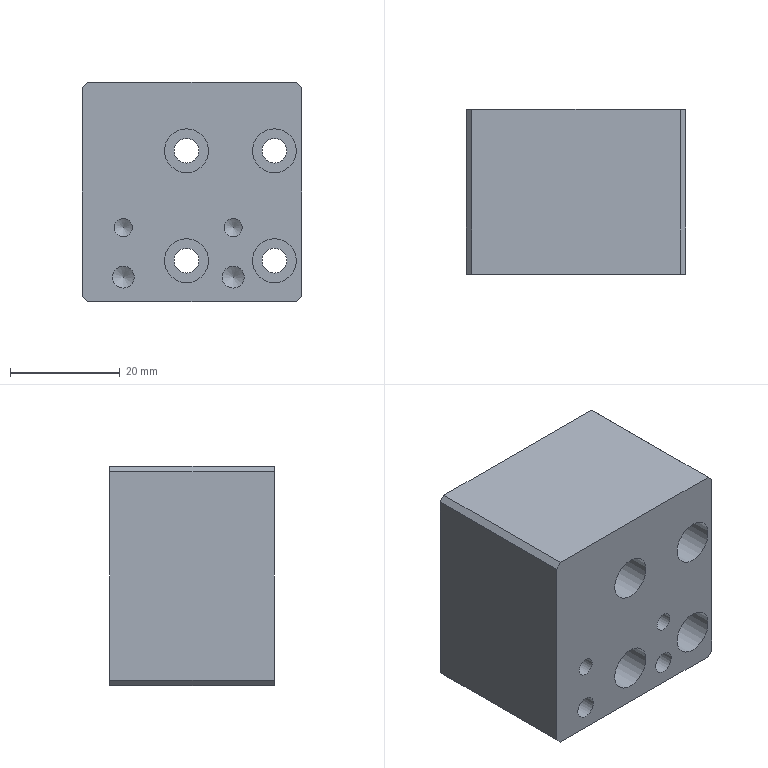Part | NX | 1 solid | 30 faces | box 40 x 30 x 40 mm | volume 42153 mm3 | plane 14 | cylinder 12 | cone 4 | commonest cylinder face diameters 4.5 x4 8 x4 3.3 x2 4 x2
STEP:
#1=CARTESIAN_POINT('',(-19.,30.,-20.));
#2=VERTEX_POINT('',#1);
#3=CARTESIAN_POINT('',(-20.,30.,-19.));
#4=VERTEX_POINT('',#3);
#5=CARTESIAN_POINT('',(-20.,30.,-19.));
#6=DIRECTION('',(-0.7071,0.,0.7071));
#7=VECTOR('',#6,1000.);
#8=LINE('',#5,#7);
#9=EDGE_CURVE('',#2,#4,#8,.T.);
#10=ORIENTED_EDGE('',*,*,#9,.F.);
#11=CARTESIAN_POINT('',(-19.,0.,-20.));
#12=VERTEX_POINT('',#11);
#13=CARTESIAN_POINT('',(-19.,30.,-20.));
#14=DIRECTION('',(0.,1.,0.));
#15=VECTOR('',#14,1000.);
#16=LINE('',#13,#15);
#17=EDGE_CURVE('',#12,#2,#16,.T.);
#18=ORIENTED_EDGE('',*,*,#17,.F.);
#19=CARTESIAN_POINT('',(-20.,0.,-19.));
#20=VERTEX_POINT('',#19);
#21=CARTESIAN_POINT('',(-19.5,0.,-19.5));
#22=DIRECTION('',(0.7071,0.,-0.7071));
#23=VECTOR('',#22,1000.);
#24=LINE('',#21,#23);
#25=EDGE_CURVE('',#20,#12,#24,.T.);
#26=ORIENTED_EDGE('',*,*,#25,.F.);
#27=CARTESIAN_POINT('',(-20.,30.,-19.));
#28=DIRECTION('',(0.,-1.,0.));
#29=VECTOR('',#28,1000.);
#30=LINE('',#27,#29);
#31=EDGE_CURVE('',#4,#20,#30,.T.);
#32=ORIENTED_EDGE('',*,*,#31,.F.);
#33=EDGE_LOOP('',(#10,#18,#26,#32));
#34=FACE_BOUND('',#33,.T.);
#35=CARTESIAN_POINT('',(-20.,30.,-19.));
#36=DIRECTION('',(0.7071,0.,0.7071));
#37=DIRECTION('',(0.,-1.,0.));
#38=AXIS2_PLACEMENT_3D('',#35,#36,#37);
#39=PLANE('',#38);
#40=ADVANCED_FACE('',(#34),#39,.F.);
#41=CARTESIAN_POINT('',(-20.,30.,19.));
#42=VERTEX_POINT('',#41);
#43=CARTESIAN_POINT('',(-19.,30.,20.));
#44=VERTEX_POINT('',#43);
#45=CARTESIAN_POINT('',(-19.,30.,20.));
#46=DIRECTION('',(0.7071,0.,0.7071));
#47=VECTOR('',#46,1000.);
#48=LINE('',#45,#47);
#49=EDGE_CURVE('',#42,#44,#48,.T.);
#50=ORIENTED_EDGE('',*,*,#49,.F.);
#51=CARTESIAN_POINT('',(-20.,0.,19.));
#52=VERTEX_POINT('',#51);
#53=CARTESIAN_POINT('',(-20.,30.,19.));
#54=DIRECTION('',(0.,1.,0.));
#55=VECTOR('',#54,1000.);
#56=LINE('',#53,#55);
#57=EDGE_CURVE('',#52,#42,#56,.T.);
#58=ORIENTED_EDGE('',*,*,#57,.F.);
#59=CARTESIAN_POINT('',(-19.,0.,20.));
#60=VERTEX_POINT('',#59);
#61=CARTESIAN_POINT('',(-19.5,0.,19.5));
#62=DIRECTION('',(-0.7071,0.,-0.7071));
#63=VECTOR('',#62,1000.);
#64=LINE('',#61,#63);
#65=EDGE_CURVE('',#60,#52,#64,.T.);
#66=ORIENTED_EDGE('',*,*,#65,.F.);
#67=CARTESIAN_POINT('',(-19.,30.,20.));
#68=DIRECTION('',(0.,-1.,0.));
#69=VECTOR('',#68,1000.);
#70=LINE('',#67,#69);
#71=EDGE_CURVE('',#44,#60,#70,.T.);
#72=ORIENTED_EDGE('',*,*,#71,.F.);
#73=EDGE_LOOP('',(#50,#58,#66,#72));
#74=FACE_BOUND('',#73,.T.);
#75=CARTESIAN_POINT('',(-19.,30.,20.));
#76=DIRECTION('',(0.7071,0.,-0.7071));
#77=DIRECTION('',(0.,-1.,0.));
#78=AXIS2_PLACEMENT_3D('',#75,#76,#77);
#79=PLANE('',#78);
#80=ADVANCED_FACE('',(#74),#79,.F.);
#81=CARTESIAN_POINT('',(19.,30.,20.));
#82=VERTEX_POINT('',#81);
#83=CARTESIAN_POINT('',(20.,30.,19.));
#84=VERTEX_POINT('',#83);
#85=CARTESIAN_POINT('',(20.,30.,19.));
#86=DIRECTION('',(0.7071,0.,-0.7071));
#87=VECTOR('',#86,1000.);
#88=LINE('',#85,#87);
#89=EDGE_CURVE('',#82,#84,#88,.T.);
#90=ORIENTED_EDGE('',*,*,#89,.F.);
#91=CARTESIAN_POINT('',(19.,0.,20.));
#92=VERTEX_POINT('',#91);
#93=CARTESIAN_POINT('',(19.,30.,20.));
#94=DIRECTION('',(0.,1.,0.));
#95=VECTOR('',#94,1000.);
#96=LINE('',#93,#95);
#97=EDGE_CURVE('',#92,#82,#96,.T.);
#98=ORIENTED_EDGE('',*,*,#97,.F.);
#99=CARTESIAN_POINT('',(20.,0.,19.));
#100=VERTEX_POINT('',#99);
#101=CARTESIAN_POINT('',(19.5,0.,19.5));
#102=DIRECTION('',(-0.7071,0.,0.7071));
#103=VECTOR('',#102,1000.);
#104=LINE('',#101,#103);
#105=EDGE_CURVE('',#100,#92,#104,.T.);
#106=ORIENTED_EDGE('',*,*,#105,.F.);
#107=CARTESIAN_POINT('',(20.,30.,19.));
#108=DIRECTION('',(0.,-1.,0.));
#109=VECTOR('',#108,1000.);
#110=LINE('',#107,#109);
#111=EDGE_CURVE('',#84,#100,#110,.T.);
#112=ORIENTED_EDGE('',*,*,#111,.F.);
#113=EDGE_LOOP('',(#90,#98,#106,#112));
#114=FACE_BOUND('',#113,.T.);
#115=CARTESIAN_POINT('',(20.,30.,19.));
#116=DIRECTION('',(-0.7071,0.,-0.7071));
#117=DIRECTION('',(0.,-1.,0.));
#118=AXIS2_PLACEMENT_3D('',#115,#116,#117);
#119=PLANE('',#118);
#120=ADVANCED_FACE('',(#114),#119,.F.);
#121=CARTESIAN_POINT('',(20.,30.,-19.));
#122=VERTEX_POINT('',#121);
#123=CARTESIAN_POINT('',(19.,30.,-20.));
#124=VERTEX_POINT('',#123);
#125=CARTESIAN_POINT('',(19.,30.,-20.));
#126=DIRECTION('',(-0.7071,0.,-0.7071));
#127=VECTOR('',#126,1000.);
#128=LINE('',#125,#127);
#129=EDGE_CURVE('',#122,#124,#128,.T.);
#130=ORIENTED_EDGE('',*,*,#129,.F.);
#131=CARTESIAN_POINT('',(20.,0.,-19.));
#132=VERTEX_POINT('',#131);
#133=CARTESIAN_POINT('',(20.,30.,-19.));
#134=DIRECTION('',(0.,1.,0.));
#135=VECTOR('',#134,1000.);
#136=LINE('',#133,#135);
#137=EDGE_CURVE('',#132,#122,#136,.T.);
#138=ORIENTED_EDGE('',*,*,#137,.F.);
#139=CARTESIAN_POINT('',(19.,0.,-20.));
#140=VERTEX_POINT('',#139);
#141=CARTESIAN_POINT('',(19.5,0.,-19.5));
#142=DIRECTION('',(0.7071,0.,0.7071));
#143=VECTOR('',#142,1000.);
#144=LINE('',#141,#143);
#145=EDGE_CURVE('',#140,#132,#144,.T.);
#146=ORIENTED_EDGE('',*,*,#145,.F.);
#147=CARTESIAN_POINT('',(19.,30.,-20.));
#148=DIRECTION('',(0.,-1.,0.));
#149=VECTOR('',#148,1000.);
#150=LINE('',#147,#149);
#151=EDGE_CURVE('',#124,#140,#150,.T.);
#152=ORIENTED_EDGE('',*,*,#151,.F.);
#153=EDGE_LOOP('',(#130,#138,#146,#152));
#154=FACE_BOUND('',#153,.T.);
#155=CARTESIAN_POINT('',(19.,30.,-20.));
#156=DIRECTION('',(-0.7071,0.,0.7071));
#157=DIRECTION('',(0.,-1.,0.));
#158=AXIS2_PLACEMENT_3D('',#155,#156,#157);
#159=PLANE('',#158);
#160=ADVANCED_FACE('',(#154),#159,.F.);
#161=CARTESIAN_POINT('',(15.,25.,-16.5));
#162=VERTEX_POINT('',#161);
#163=CARTESIAN_POINT('',(15.,25.,-12.5));
#164=DIRECTION('',(0.,-1.,0.));
#165=DIRECTION('',(0.,0.,-1.));
#166=AXIS2_PLACEMENT_3D('',#163,#164,#165);
#167=CIRCLE('',#166,4.);
#168=EDGE_CURVE('',#162,#162,#167,.T.);
#169=ORIENTED_EDGE('',*,*,#168,.T.);
#170=EDGE_LOOP('',(#169));
#171=FACE_BOUND('',#170,.T.);
#172=CARTESIAN_POINT('',(15.,25.,-14.75));
#173=VERTEX_POINT('',#172);
#174=CARTESIAN_POINT('',(15.,25.,-12.5));
#175=DIRECTION('',(0.,-1.,0.));
#176=DIRECTION('',(0.,0.,-1.));
#177=AXIS2_PLACEMENT_3D('',#174,#175,#176);
#178=CIRCLE('',#177,2.25);
#179=EDGE_CURVE('',#173,#173,#178,.T.);
#180=ORIENTED_EDGE('',*,*,#179,.F.);
#181=EDGE_LOOP('',(#180));
#182=FACE_BOUND('',#181,.T.);
#183=CARTESIAN_POINT('',(17.25,25.,-12.5));
#184=DIRECTION('',(0.,1.,0.));
#185=DIRECTION('',(0.,0.,1.));
#186=AXIS2_PLACEMENT_3D('',#183,#184,#185);
#187=PLANE('',#186);
#188=ADVANCED_FACE('',(#171,#182),#187,.F.);
#189=CARTESIAN_POINT('',(-1.,25.,-8.5));
#190=VERTEX_POINT('',#189);
#191=CARTESIAN_POINT('',(-1.,25.,-12.5));
#192=DIRECTION('',(0.,-1.,0.));
#193=DIRECTION('',(0.,0.,1.));
#194=AXIS2_PLACEMENT_3D('',#191,#192,#193);
#195=CIRCLE('',#194,4.);
#196=EDGE_CURVE('',#190,#190,#195,.T.);
#197=ORIENTED_EDGE('',*,*,#196,.T.);
#198=EDGE_LOOP('',(#197));
#199=FACE_BOUND('',#198,.T.);
#200=CARTESIAN_POINT('',(-1.,25.,-10.25));
#201=VERTEX_POINT('',#200);
#202=CARTESIAN_POINT('',(-1.,25.,-12.5));
#203=DIRECTION('',(0.,-1.,0.));
#204=DIRECTION('',(0.,0.,1.));
#205=AXIS2_PLACEMENT_3D('',#202,#203,#204);
#206=CIRCLE('',#205,2.25);
#207=EDGE_CURVE('',#201,#201,#206,.T.);
#208=ORIENTED_EDGE('',*,*,#207,.F.);
#209=EDGE_LOOP('',(#208));
#210=FACE_BOUND('',#209,.T.);
#211=CARTESIAN_POINT('',(17.25,25.,-12.5));
#212=DIRECTION('',(0.,1.,0.));
#213=DIRECTION('',(0.,0.,1.));
#214=AXIS2_PLACEMENT_3D('',#211,#212,#213);
#215=PLANE('',#214);
#216=ADVANCED_FACE('',(#199,#210),#215,.F.);
#217=CARTESIAN_POINT('',(15.,25.,11.5));
#218=VERTEX_POINT('',#217);
#219=CARTESIAN_POINT('',(15.,25.,7.5));
#220=DIRECTION('',(0.,-1.,0.));
#221=DIRECTION('',(0.,0.,1.));
#222=AXIS2_PLACEMENT_3D('',#219,#220,#221);
#223=CIRCLE('',#222,4.);
#224=EDGE_CURVE('',#218,#218,#223,.T.);
#225=ORIENTED_EDGE('',*,*,#224,.T.);
#226=EDGE_LOOP('',(#225));
#227=FACE_BOUND('',#226,.T.);
#228=CARTESIAN_POINT('',(15.,25.,9.75));
#229=VERTEX_POINT('',#228);
#230=CARTESIAN_POINT('',(15.,25.,7.5));
#231=DIRECTION('',(0.,-1.,0.));
#232=DIRECTION('',(0.,0.,1.));
#233=AXIS2_PLACEMENT_3D('',#230,#231,#232);
#234=CIRCLE('',#233,2.25);
#235=EDGE_CURVE('',#229,#229,#234,.T.);
#236=ORIENTED_EDGE('',*,*,#235,.F.);
#237=EDGE_LOOP('',(#236));
#238=FACE_BOUND('',#237,.T.);
#239=CARTESIAN_POINT('',(17.25,25.,-12.5));
#240=DIRECTION('',(0.,1.,0.));
#241=DIRECTION('',(0.,0.,1.));
#242=AXIS2_PLACEMENT_3D('',#239,#240,#241);
#243=PLANE('',#242);
#244=ADVANCED_FACE('',(#227,#238),#243,.F.);
#245=CARTESIAN_POINT('',(-1.,25.,11.5));
#246=VERTEX_POINT('',#245);
#247=CARTESIAN_POINT('',(-1.,25.,7.5));
#248=DIRECTION('',(0.,-1.,0.));
#249=DIRECTION('',(0.,0.,1.));
#250=AXIS2_PLACEMENT_3D('',#247,#248,#249);
#251=CIRCLE('',#250,4.);
#252=EDGE_CURVE('',#246,#246,#251,.T.);
#253=ORIENTED_EDGE('',*,*,#252,.T.);
#254=EDGE_LOOP('',(#253));
#255=FACE_BOUND('',#254,.T.);
#256=CARTESIAN_POINT('',(-1.,25.,9.75));
#257=VERTEX_POINT('',#256);
#258=CARTESIAN_POINT('',(-1.,25.,7.5));
#259=DIRECTION('',(0.,-1.,0.));
#260=DIRECTION('',(0.,0.,1.));
#261=AXIS2_PLACEMENT_3D('',#258,#259,#260);
#262=CIRCLE('',#261,2.25);
#263=EDGE_CURVE('',#257,#257,#262,.T.);
#264=ORIENTED_EDGE('',*,*,#263,.F.);
#265=EDGE_LOOP('',(#264));
#266=FACE_BOUND('',#265,.T.);
#267=CARTESIAN_POINT('',(17.25,25.,-12.5));
#268=DIRECTION('',(0.,1.,0.));
#269=DIRECTION('',(0.,0.,1.));
#270=AXIS2_PLACEMENT_3D('',#267,#268,#269);
#271=PLANE('',#270);
#272=ADVANCED_FACE('',(#255,#266),#271,.F.);
#273=CARTESIAN_POINT('',(-20.,0.,-20.));
#274=DIRECTION('',(-1.,0.,0.));
#275=VECTOR('',#274,1000.);
#276=LINE('',#273,#275);
#277=EDGE_CURVE('',#140,#12,#276,.T.);
#278=ORIENTED_EDGE('',*,*,#277,.F.);
#279=ORIENTED_EDGE('',*,*,#145,.T.);
#280=CARTESIAN_POINT('',(20.,0.,20.));
#281=DIRECTION('',(0.,0.,-1.));
#282=VECTOR('',#281,1000.);
#283=LINE('',#280,#282);
#284=EDGE_CURVE('',#100,#132,#283,.T.);
#285=ORIENTED_EDGE('',*,*,#284,.F.);
#286=ORIENTED_EDGE('',*,*,#105,.T.);
#287=CARTESIAN_POINT('',(-20.,0.,20.));
#288=DIRECTION('',(1.,0.,0.));
#289=VECTOR('',#288,1000.);
#290=LINE('',#287,#289);
#291=EDGE_CURVE('',#60,#92,#290,.T.);
#292=ORIENTED_EDGE('',*,*,#291,.F.);
#293=ORIENTED_EDGE('',*,*,#65,.T.);
#294=CARTESIAN_POINT('',(-20.,0.,20.));
#295=DIRECTION('',(0.,0.,1.));
#296=VECTOR('',#295,1000.);
#297=LINE('',#294,#296);
#298=EDGE_CURVE('',#20,#52,#297,.T.);
#299=ORIENTED_EDGE('',*,*,#298,.F.);
#300=ORIENTED_EDGE('',*,*,#25,.T.);
#301=EDGE_LOOP('',(#278,#279,#285,#286,#292,#293,#299,#300));
#302=FACE_BOUND('',#301,.T.);
#303=CARTESIAN_POINT('',(-1.,0.,3.5));
#304=VERTEX_POINT('',#303);
#305=CARTESIAN_POINT('',(-1.,0.,7.5));
#306=DIRECTION('',(0.,-1.,0.));
#307=DIRECTION('',(0.,0.,-1.));
#308=AXIS2_PLACEMENT_3D('',#305,#306,#307);
#309=CIRCLE('',#308,4.);
#310=EDGE_CURVE('',#304,#304,#309,.T.);
#311=ORIENTED_EDGE('',*,*,#310,.F.);
#312=EDGE_LOOP('',(#311));
#313=FACE_BOUND('',#312,.T.);
#314=CARTESIAN_POINT('',(15.,0.,3.5));
#315=VERTEX_POINT('',#314);
#316=CARTESIAN_POINT('',(15.,0.,7.5));
#317=DIRECTION('',(0.,-1.,0.));
#318=DIRECTION('',(0.,0.,-1.));
#319=AXIS2_PLACEMENT_3D('',#316,#317,#318);
#320=CIRCLE('',#319,4.);
#321=EDGE_CURVE('',#315,#315,#320,.T.);
#322=ORIENTED_EDGE('',*,*,#321,.F.);
#323=EDGE_LOOP('',(#322));
#324=FACE_BOUND('',#323,.T.);
#325=CARTESIAN_POINT('',(-1.,0.,-16.5));
#326=VERTEX_POINT('',#325);
#327=CARTESIAN_POINT('',(-1.,0.,-12.5));
#328=DIRECTION('',(0.,-1.,0.));
#329=DIRECTION('',(0.,0.,-1.));
#330=AXIS2_PLACEMENT_3D('',#327,#328,#329);
#331=CIRCLE('',#330,4.);
#332=EDGE_CURVE('',#326,#326,#331,.T.);
#333=ORIENTED_EDGE('',*,*,#332,.F.);
#334=EDGE_LOOP('',(#333));
#335=FACE_BOUND('',#334,.T.);
#336=CARTESIAN_POINT('',(15.,0.,-16.5));
#337=VERTEX_POINT('',#336);
#338=CARTESIAN_POINT('',(15.,0.,-12.5));
#339=DIRECTION('',(0.,-1.,0.));
#340=DIRECTION('',(0.,0.,-1.));
#341=AXIS2_PLACEMENT_3D('',#338,#339,#340);
#342=CIRCLE('',#341,4.);
#343=EDGE_CURVE('',#337,#337,#342,.T.);
#344=ORIENTED_EDGE('',*,*,#343,.F.);
#345=EDGE_LOOP('',(#344));
#346=FACE_BOUND('',#345,.T.);
#347=CARTESIAN_POINT('',(-12.5,0.,-8.15));
#348=VERTEX_POINT('',#347);
#349=CARTESIAN_POINT('',(-12.5,0.,-6.5));
#350=DIRECTION('',(0.,-1.,0.));
#351=DIRECTION('',(0.,0.,-1.));
#352=AXIS2_PLACEMENT_3D('',#349,#350,#351);
#353=CIRCLE('',#352,1.65);
#354=EDGE_CURVE('',#348,#348,#353,.T.);
#355=ORIENTED_EDGE('',*,*,#354,.F.);
#356=EDGE_LOOP('',(#355));
#357=FACE_BOUND('',#356,.T.);
#358=CARTESIAN_POINT('',(7.5,0.,-8.15));
#359=VERTEX_POINT('',#358);
#360=CARTESIAN_POINT('',(7.5,0.,-6.5));
#361=DIRECTION('',(0.,-1.,0.));
#362=DIRECTION('',(0.,0.,-1.));
#363=AXIS2_PLACEMENT_3D('',#360,#361,#362);
#364=CIRCLE('',#363,1.65);
#365=EDGE_CURVE('',#359,#359,#364,.T.);
#366=ORIENTED_EDGE('',*,*,#365,.F.);
#367=EDGE_LOOP('',(#366));
#368=FACE_BOUND('',#367,.T.);
#369=CARTESIAN_POINT('',(-12.5,0.,-17.5));
#370=VERTEX_POINT('',#369);
#371=CARTESIAN_POINT('',(-12.5,0.,-15.5));
#372=DIRECTION('',(0.,-1.,0.));
#373=DIRECTION('',(0.,0.,-1.));
#374=AXIS2_PLACEMENT_3D('',#371,#372,#373);
#375=CIRCLE('',#374,2.);
#376=EDGE_CURVE('',#370,#370,#375,.T.);
#377=ORIENTED_EDGE('',*,*,#376,.F.);
#378=EDGE_LOOP('',(#377));
#379=FACE_BOUND('',#378,.T.);
#380=CARTESIAN_POINT('',(7.5,0.,-17.5));
#381=VERTEX_POINT('',#380);
#382=CARTESIAN_POINT('',(7.5,0.,-15.5));
#383=DIRECTION('',(0.,-1.,0.));
#384=DIRECTION('',(0.,0.,-1.));
#385=AXIS2_PLACEMENT_3D('',#382,#383,#384);
#386=CIRCLE('',#385,2.);
#387=EDGE_CURVE('',#381,#381,#386,.T.);
#388=ORIENTED_EDGE('',*,*,#387,.F.);
#389=EDGE_LOOP('',(#388));
#390=FACE_BOUND('',#389,.T.);
#391=CARTESIAN_POINT('',(0.,0.,0.));
#392=DIRECTION('',(0.,-1.,0.));
#393=DIRECTION('',(0.,0.,-1.));
#394=AXIS2_PLACEMENT_3D('',#391,#392,#393);
#395=PLANE('',#394);
#396=ADVANCED_FACE('',(#302,#313,#324,#335,#346,#357,#368,#379,#390),#395,.T.);
#397=CARTESIAN_POINT('',(20.,30.,20.));
#398=DIRECTION('',(0.,0.,-1.));
#399=VECTOR('',#398,1000.);
#400=LINE('',#397,#399);
#401=EDGE_CURVE('',#84,#122,#400,.T.);
#402=ORIENTED_EDGE('',*,*,#401,.T.);
#403=ORIENTED_EDGE('',*,*,#129,.T.);
#404=CARTESIAN_POINT('',(-20.,30.,-20.));
#405=DIRECTION('',(-1.,0.,0.));
#406=VECTOR('',#405,1000.);
#407=LINE('',#404,#406);
#408=EDGE_CURVE('',#124,#2,#407,.T.);
#409=ORIENTED_EDGE('',*,*,#408,.T.);
#410=ORIENTED_EDGE('',*,*,#9,.T.);
#411=CARTESIAN_POINT('',(-20.,30.,20.));
#412=DIRECTION('',(0.,0.,1.));
#413=VECTOR('',#412,1000.);
#414=LINE('',#411,#413);
#415=EDGE_CURVE('',#4,#42,#414,.T.);
#416=ORIENTED_EDGE('',*,*,#415,.T.);
#417=ORIENTED_EDGE('',*,*,#49,.T.);
#418=CARTESIAN_POINT('',(-20.,30.,20.));
#419=DIRECTION('',(1.,0.,0.));
#420=VECTOR('',#419,1000.);
#421=LINE('',#418,#420);
#422=EDGE_CURVE('',#44,#82,#421,.T.);
#423=ORIENTED_EDGE('',*,*,#422,.T.);
#424=ORIENTED_EDGE('',*,*,#89,.T.);
#425=EDGE_LOOP('',(#402,#403,#409,#410,#416,#417,#423,#424));
#426=FACE_BOUND('',#425,.T.);
#427=CARTESIAN_POINT('',(-1.,30.,5.25));
#428=VERTEX_POINT('',#427);
#429=CARTESIAN_POINT('',(-1.,30.,7.5));
#430=DIRECTION('',(0.,-1.,0.));
#431=DIRECTION('',(0.,0.,-1.));
#432=AXIS2_PLACEMENT_3D('',#429,#430,#431);
#433=CIRCLE('',#432,2.25);
#434=EDGE_CURVE('',#428,#428,#433,.T.);
#435=ORIENTED_EDGE('',*,*,#434,.T.);
#436=EDGE_LOOP('',(#435));
#437=FACE_BOUND('',#436,.T.);
#438=CARTESIAN_POINT('',(15.,30.,5.25));
#439=VERTEX_POINT('',#438);
#440=CARTESIAN_POINT('',(15.,30.,7.5));
#441=DIRECTION('',(0.,-1.,0.));
#442=DIRECTION('',(0.,0.,-1.));
#443=AXIS2_PLACEMENT_3D('',#440,#441,#442);
#444=CIRCLE('',#443,2.25);
#445=EDGE_CURVE('',#439,#439,#444,.T.);
#446=ORIENTED_EDGE('',*,*,#445,.T.);
#447=EDGE_LOOP('',(#446));
#448=FACE_BOUND('',#447,.T.);
#449=CARTESIAN_POINT('',(-1.,30.,-14.75));
#450=VERTEX_POINT('',#449);
#451=CARTESIAN_POINT('',(-1.,30.,-12.5));
#452=DIRECTION('',(0.,-1.,0.));
#453=DIRECTION('',(0.,0.,-1.));
#454=AXIS2_PLACEMENT_3D('',#451,#452,#453);
#455=CIRCLE('',#454,2.25);
#456=EDGE_CURVE('',#450,#450,#455,.T.);
#457=ORIENTED_EDGE('',*,*,#456,.T.);
#458=EDGE_LOOP('',(#457));
#459=FACE_BOUND('',#458,.T.);
#460=CARTESIAN_POINT('',(15.,30.,-14.75));
#461=VERTEX_POINT('',#460);
#462=CARTESIAN_POINT('',(15.,30.,-12.5));
#463=DIRECTION('',(0.,-1.,0.));
#464=DIRECTION('',(0.,0.,-1.));
#465=AXIS2_PLACEMENT_3D('',#462,#463,#464);
#466=CIRCLE('',#465,2.25);
#467=EDGE_CURVE('',#461,#461,#466,.T.);
#468=ORIENTED_EDGE('',*,*,#467,.T.);
#469=EDGE_LOOP('',(#468));
#470=FACE_BOUND('',#469,.T.);
#471=CARTESIAN_POINT('',(0.,30.,0.));
#472=DIRECTION('',(0.,-1.,0.));
#473=DIRECTION('',(0.,0.,-1.));
#474=AXIS2_PLACEMENT_3D('',#471,#472,#473);
#475=PLANE('',#474);
#476=ADVANCED_FACE('',(#426,#437,#448,#459,#470),#475,.F.);
#477=ORIENTED_EDGE('',*,*,#291,.T.);
#478=ORIENTED_EDGE('',*,*,#97,.T.);
#479=ORIENTED_EDGE('',*,*,#422,.F.);
#480=ORIENTED_EDGE('',*,*,#71,.T.);
#481=EDGE_LOOP('',(#477,#478,#479,#480));
#482=FACE_BOUND('',#481,.T.);
#483=CARTESIAN_POINT('',(-20.,30.,20.));
#484=DIRECTION('',(0.,0.,-1.));
#485=DIRECTION('',(-1.,0.,0.));
#486=AXIS2_PLACEMENT_3D('',#483,#484,#485);
#487=PLANE('',#486);
#488=ADVANCED_FACE('',(#482),#487,.F.);
#489=ORIENTED_EDGE('',*,*,#298,.T.);
#490=ORIENTED_EDGE('',*,*,#57,.T.);
#491=ORIENTED_EDGE('',*,*,#415,.F.);
#492=ORIENTED_EDGE('',*,*,#31,.T.);
#493=EDGE_LOOP('',(#489,#490,#491,#492));
#494=FACE_BOUND('',#493,.T.);
#495=CARTESIAN_POINT('',(-20.,30.,20.));
#496=DIRECTION('',(1.,0.,0.));
#497=DIRECTION('',(0.,0.,-1.));
#498=AXIS2_PLACEMENT_3D('',#495,#496,#497);
#499=PLANE('',#498);
#500=ADVANCED_FACE('',(#494),#499,.F.);
#501=ORIENTED_EDGE('',*,*,#408,.F.);
#502=ORIENTED_EDGE('',*,*,#151,.T.);
#503=ORIENTED_EDGE('',*,*,#277,.T.);
#504=ORIENTED_EDGE('',*,*,#17,.T.);
#505=EDGE_LOOP('',(#501,#502,#503,#504));
#506=FACE_BOUND('',#505,.T.);
#507=CARTESIAN_POINT('',(-20.,30.,-20.));
#508=DIRECTION('',(0.,0.,1.));
#509=DIRECTION('',(1.,0.,0.));
#510=AXIS2_PLACEMENT_3D('',#507,#508,#509);
#511=PLANE('',#510);
#512=ADVANCED_FACE('',(#506),#511,.F.);
#513=ORIENTED_EDGE('',*,*,#284,.T.);
#514=ORIENTED_EDGE('',*,*,#137,.T.);
#515=ORIENTED_EDGE('',*,*,#401,.F.);
#516=ORIENTED_EDGE('',*,*,#111,.T.);
#517=EDGE_LOOP('',(#513,#514,#515,#516));
#518=FACE_BOUND('',#517,.T.);
#519=CARTESIAN_POINT('',(20.,30.,20.));
#520=DIRECTION('',(-1.,0.,0.));
#521=DIRECTION('',(0.,0.,1.));
#522=AXIS2_PLACEMENT_3D('',#519,#520,#521);
#523=PLANE('',#522);
#524=ADVANCED_FACE('',(#518),#523,.F.);
#525=ORIENTED_EDGE('',*,*,#263,.T.);
#526=EDGE_LOOP('',(#525));
#527=FACE_BOUND('',#526,.T.);
#528=ORIENTED_EDGE('',*,*,#434,.F.);
#529=EDGE_LOOP('',(#528));
#530=FACE_BOUND('',#529,.T.);
#531=CARTESIAN_POINT('',(-1.,0.,7.5));
#532=DIRECTION('',(0.,-1.,0.));
#533=DIRECTION('',(0.,0.,-1.));
#534=AXIS2_PLACEMENT_3D('',#531,#532,#533);
#535=CYLINDRICAL_SURFACE('',#534,2.25);
#536=ADVANCED_FACE('',(#527,#530),#535,.F.);
#537=ORIENTED_EDGE('',*,*,#310,.T.);
#538=EDGE_LOOP('',(#537));
#539=FACE_BOUND('',#538,.T.);
#540=ORIENTED_EDGE('',*,*,#252,.F.);
#541=EDGE_LOOP('',(#540));
#542=FACE_BOUND('',#541,.T.);
#543=CARTESIAN_POINT('',(-1.,0.,7.5));
#544=DIRECTION('',(0.,-1.,0.));
#545=DIRECTION('',(0.,0.,-1.));
#546=AXIS2_PLACEMENT_3D('',#543,#544,#545);
#547=CYLINDRICAL_SURFACE('',#546,4.);
#548=ADVANCED_FACE('',(#539,#542),#547,.F.);
#549=ORIENTED_EDGE('',*,*,#235,.T.);
#550=EDGE_LOOP('',(#549));
#551=FACE_BOUND('',#550,.T.);
#552=ORIENTED_EDGE('',*,*,#445,.F.);
#553=EDGE_LOOP('',(#552));
#554=FACE_BOUND('',#553,.T.);
#555=CARTESIAN_POINT('',(15.,0.,7.5));
#556=DIRECTION('',(0.,-1.,0.));
#557=DIRECTION('',(0.,0.,-1.));
#558=AXIS2_PLACEMENT_3D('',#555,#556,#557);
#559=CYLINDRICAL_SURFACE('',#558,2.25);
#560=ADVANCED_FACE('',(#551,#554),#559,.F.);
#561=ORIENTED_EDGE('',*,*,#321,.T.);
#562=EDGE_LOOP('',(#561));
#563=FACE_BOUND('',#562,.T.);
#564=ORIENTED_EDGE('',*,*,#224,.F.);
#565=EDGE_LOOP('',(#564));
#566=FACE_BOUND('',#565,.T.);
#567=CARTESIAN_POINT('',(15.,0.,7.5));
#568=DIRECTION('',(0.,-1.,0.));
#569=DIRECTION('',(0.,0.,-1.));
#570=AXIS2_PLACEMENT_3D('',#567,#568,#569);
#571=CYLINDRICAL_SURFACE('',#570,4.);
#572=ADVANCED_FACE('',(#563,#566),#571,.F.);
#573=ORIENTED_EDGE('',*,*,#207,.T.);
#574=EDGE_LOOP('',(#573));
#575=FACE_BOUND('',#574,.T.);
#576=ORIENTED_EDGE('',*,*,#456,.F.);
#577=EDGE_LOOP('',(#576));
#578=FACE_BOUND('',#577,.T.);
#579=CARTESIAN_POINT('',(-1.,0.,-12.5));
#580=DIRECTION('',(0.,-1.,0.));
#581=DIRECTION('',(0.,0.,-1.));
#582=AXIS2_PLACEMENT_3D('',#579,#580,#581);
#583=CYLINDRICAL_SURFACE('',#582,2.25);
#584=ADVANCED_FACE('',(#575,#578),#583,.F.);
#585=ORIENTED_EDGE('',*,*,#332,.T.);
#586=EDGE_LOOP('',(#585));
#587=FACE_BOUND('',#586,.T.);
#588=ORIENTED_EDGE('',*,*,#196,.F.);
#589=EDGE_LOOP('',(#588));
#590=FACE_BOUND('',#589,.T.);
#591=CARTESIAN_POINT('',(-1.,0.,-12.5));
#592=DIRECTION('',(0.,-1.,0.));
#593=DIRECTION('',(0.,0.,-1.));
#594=AXIS2_PLACEMENT_3D('',#591,#592,#593);
#595=CYLINDRICAL_SURFACE('',#594,4.);
#596=ADVANCED_FACE('',(#587,#590),#595,.F.);
#597=ORIENTED_EDGE('',*,*,#179,.T.);
#598=EDGE_LOOP('',(#597));
#599=FACE_BOUND('',#598,.T.);
#600=ORIENTED_EDGE('',*,*,#467,.F.);
#601=EDGE_LOOP('',(#600));
#602=FACE_BOUND('',#601,.T.);
#603=CARTESIAN_POINT('',(15.,0.,-12.5));
#604=DIRECTION('',(0.,-1.,0.));
#605=DIRECTION('',(0.,0.,-1.));
#606=AXIS2_PLACEMENT_3D('',#603,#604,#605);
#607=CYLINDRICAL_SURFACE('',#606,2.25);
#608=ADVANCED_FACE('',(#599,#602),#607,.F.);
#609=ORIENTED_EDGE('',*,*,#343,.T.);
#610=EDGE_LOOP('',(#609));
#611=FACE_BOUND('',#610,.T.);
#612=ORIENTED_EDGE('',*,*,#168,.F.);
#613=EDGE_LOOP('',(#612));
#614=FACE_BOUND('',#613,.T.);
#615=CARTESIAN_POINT('',(15.,0.,-12.5));
#616=DIRECTION('',(0.,-1.,0.));
#617=DIRECTION('',(0.,0.,-1.));
#618=AXIS2_PLACEMENT_3D('',#615,#616,#617);
#619=CYLINDRICAL_SURFACE('',#618,4.);
#620=ADVANCED_FACE('',(#611,#614),#619,.F.);
#621=CARTESIAN_POINT('',(-12.5,11.091,-6.5));
#622=VERTEX_POINT('',#621);
#623=VERTEX_LOOP('',#622);
#624=FACE_BOUND('',#623,.T.);
#625=CARTESIAN_POINT('',(-12.5,10.1,-8.15));
#626=VERTEX_POINT('',#625);
#627=CARTESIAN_POINT('',(-12.5,10.1,-6.5));
#628=DIRECTION('',(0.,-1.,0.));
#629=DIRECTION('',(0.,0.,-1.));
#630=AXIS2_PLACEMENT_3D('',#627,#628,#629);
#631=CIRCLE('',#630,1.65);
#632=EDGE_CURVE('',#626,#626,#631,.T.);
#633=ORIENTED_EDGE('',*,*,#632,.T.);
#634=EDGE_LOOP('',(#633));
#635=FACE_BOUND('',#634,.T.);
#636=CARTESIAN_POINT('',(-12.5,10.1,-6.5));
#637=DIRECTION('',(0.,-1.,0.));
#638=DIRECTION('',(0.,0.,-1.));
#639=AXIS2_PLACEMENT_3D('',#636,#637,#638);
#640=CONICAL_SURFACE('',#639,1.65,1.03);
#641=ADVANCED_FACE('',(#624,#635),#640,.F.);
#642=ORIENTED_EDGE('',*,*,#354,.T.);
#643=EDGE_LOOP('',(#642));
#644=FACE_BOUND('',#643,.T.);
#645=ORIENTED_EDGE('',*,*,#632,.F.);
#646=EDGE_LOOP('',(#645));
#647=FACE_BOUND('',#646,.T.);
#648=CARTESIAN_POINT('',(-12.5,0.,-6.5));
#649=DIRECTION('',(0.,-1.,0.));
#650=DIRECTION('',(0.,0.,-1.));
#651=AXIS2_PLACEMENT_3D('',#648,#649,#650);
#652=CYLINDRICAL_SURFACE('',#651,1.65);
#653=ADVANCED_FACE('',(#644,#647),#652,.F.);
#654=CARTESIAN_POINT('',(7.5,11.091,-6.5));
#655=VERTEX_POINT('',#654);
#656=VERTEX_LOOP('',#655);
#657=FACE_BOUND('',#656,.T.);
#658=CARTESIAN_POINT('',(7.5,10.1,-8.15));
#659=VERTEX_POINT('',#658);
#660=CARTESIAN_POINT('',(7.5,10.1,-6.5));
#661=DIRECTION('',(0.,-1.,0.));
#662=DIRECTION('',(0.,0.,-1.));
#663=AXIS2_PLACEMENT_3D('',#660,#661,#662);
#664=CIRCLE('',#663,1.65);
#665=EDGE_CURVE('',#659,#659,#664,.T.);
#666=ORIENTED_EDGE('',*,*,#665,.T.);
#667=EDGE_LOOP('',(#666));
#668=FACE_BOUND('',#667,.T.);
#669=CARTESIAN_POINT('',(7.5,10.1,-6.5));
#670=DIRECTION('',(0.,-1.,0.));
#671=DIRECTION('',(0.,0.,-1.));
#672=AXIS2_PLACEMENT_3D('',#669,#670,#671);
#673=CONICAL_SURFACE('',#672,1.65,1.03);
#674=ADVANCED_FACE('',(#657,#668),#673,.F.);
#675=ORIENTED_EDGE('',*,*,#365,.T.);
#676=EDGE_LOOP('',(#675));
#677=FACE_BOUND('',#676,.T.);
#678=ORIENTED_EDGE('',*,*,#665,.F.);
#679=EDGE_LOOP('',(#678));
#680=FACE_BOUND('',#679,.T.);
#681=CARTESIAN_POINT('',(7.5,0.,-6.5));
#682=DIRECTION('',(0.,-1.,0.));
#683=DIRECTION('',(0.,0.,-1.));
#684=AXIS2_PLACEMENT_3D('',#681,#682,#683);
#685=CYLINDRICAL_SURFACE('',#684,1.65);
#686=ADVANCED_FACE('',(#677,#680),#685,.F.);
#687=CARTESIAN_POINT('',(-12.5,11.302,-15.5));
#688=VERTEX_POINT('',#687);
#689=VERTEX_LOOP('',#688);
#690=FACE_BOUND('',#689,.T.);
#691=CARTESIAN_POINT('',(-12.5,10.1,-17.5));
#692=VERTEX_POINT('',#691);
#693=CARTESIAN_POINT('',(-12.5,10.1,-15.5));
#694=DIRECTION('',(0.,-1.,0.));
#695=DIRECTION('',(0.,0.,-1.));
#696=AXIS2_PLACEMENT_3D('',#693,#694,#695);
#697=CIRCLE('',#696,2.);
#698=EDGE_CURVE('',#692,#692,#697,.T.);
#699=ORIENTED_EDGE('',*,*,#698,.T.);
#700=EDGE_LOOP('',(#699));
#701=FACE_BOUND('',#700,.T.);
#702=CARTESIAN_POINT('',(-12.5,10.1,-15.5));
#703=DIRECTION('',(0.,-1.,0.));
#704=DIRECTION('',(0.,0.,-1.));
#705=AXIS2_PLACEMENT_3D('',#702,#703,#704);
#706=CONICAL_SURFACE('',#705,2.,1.03);
#707=ADVANCED_FACE('',(#690,#701),#706,.F.);
#708=ORIENTED_EDGE('',*,*,#376,.T.);
#709=EDGE_LOOP('',(#708));
#710=FACE_BOUND('',#709,.T.);
#711=ORIENTED_EDGE('',*,*,#698,.F.);
#712=EDGE_LOOP('',(#711));
#713=FACE_BOUND('',#712,.T.);
#714=CARTESIAN_POINT('',(-12.5,0.,-15.5));
#715=DIRECTION('',(0.,-1.,0.));
#716=DIRECTION('',(0.,0.,-1.));
#717=AXIS2_PLACEMENT_3D('',#714,#715,#716);
#718=CYLINDRICAL_SURFACE('',#717,2.);
#719=ADVANCED_FACE('',(#710,#713),#718,.F.);
#720=CARTESIAN_POINT('',(7.5,11.302,-15.5));
#721=VERTEX_POINT('',#720);
#722=VERTEX_LOOP('',#721);
#723=FACE_BOUND('',#722,.T.);
#724=CARTESIAN_POINT('',(7.5,10.1,-17.5));
#725=VERTEX_POINT('',#724);
#726=CARTESIAN_POINT('',(7.5,10.1,-15.5));
#727=DIRECTION('',(0.,-1.,0.));
#728=DIRECTION('',(0.,0.,-1.));
#729=AXIS2_PLACEMENT_3D('',#726,#727,#728);
#730=CIRCLE('',#729,2.);
#731=EDGE_CURVE('',#725,#725,#730,.T.);
#732=ORIENTED_EDGE('',*,*,#731,.T.);
#733=EDGE_LOOP('',(#732));
#734=FACE_BOUND('',#733,.T.);
#735=CARTESIAN_POINT('',(7.5,10.1,-15.5));
#736=DIRECTION('',(0.,-1.,0.));
#737=DIRECTION('',(0.,0.,-1.));
#738=AXIS2_PLACEMENT_3D('',#735,#736,#737);
#739=CONICAL_SURFACE('',#738,2.,1.03);
#740=ADVANCED_FACE('',(#723,#734),#739,.F.);
#741=ORIENTED_EDGE('',*,*,#387,.T.);
#742=EDGE_LOOP('',(#741));
#743=FACE_BOUND('',#742,.T.);
#744=ORIENTED_EDGE('',*,*,#731,.F.);
#745=EDGE_LOOP('',(#744));
#746=FACE_BOUND('',#745,.T.);
#747=CARTESIAN_POINT('',(7.5,0.,-15.5));
#748=DIRECTION('',(0.,-1.,0.));
#749=DIRECTION('',(0.,0.,-1.));
#750=AXIS2_PLACEMENT_3D('',#747,#748,#749);
#751=CYLINDRICAL_SURFACE('',#750,2.);
#752=ADVANCED_FACE('',(#743,#746),#751,.F.);
#753=CLOSED_SHELL('',(#40,#80,#120,#160,#188,#216,#244,#272,#396,#476,#488,#500,#512,#524,#536,#548,#560,#572,#584,#596,#608,#620,#641,#653,#674,#686,#707,#719,#740,#752));
#754=MANIFOLD_SOLID_BREP('',#753);
#755=(LENGTH_UNIT()NAMED_UNIT(*)SI_UNIT(.MILLI.,.METRE.));
#756=UNCERTAINTY_MEASURE_WITH_UNIT(LENGTH_MEASURE(0.00001),#755,'','');
#757=(NAMED_UNIT(*)PLANE_ANGLE_UNIT()SI_UNIT($,.RADIAN.));
#758=(NAMED_UNIT(*)SI_UNIT($,.STERADIAN.)SOLID_ANGLE_UNIT());
#759=(GEOMETRIC_REPRESENTATION_CONTEXT(3)GLOBAL_UNCERTAINTY_ASSIGNED_CONTEXT((#756))GLOBAL_UNIT_ASSIGNED_CONTEXT((#755,#757,#758))REPRESENTATION_CONTEXT('',''));
#760=ADVANCED_BREP_SHAPE_REPRESENTATION('',(#754),#759);